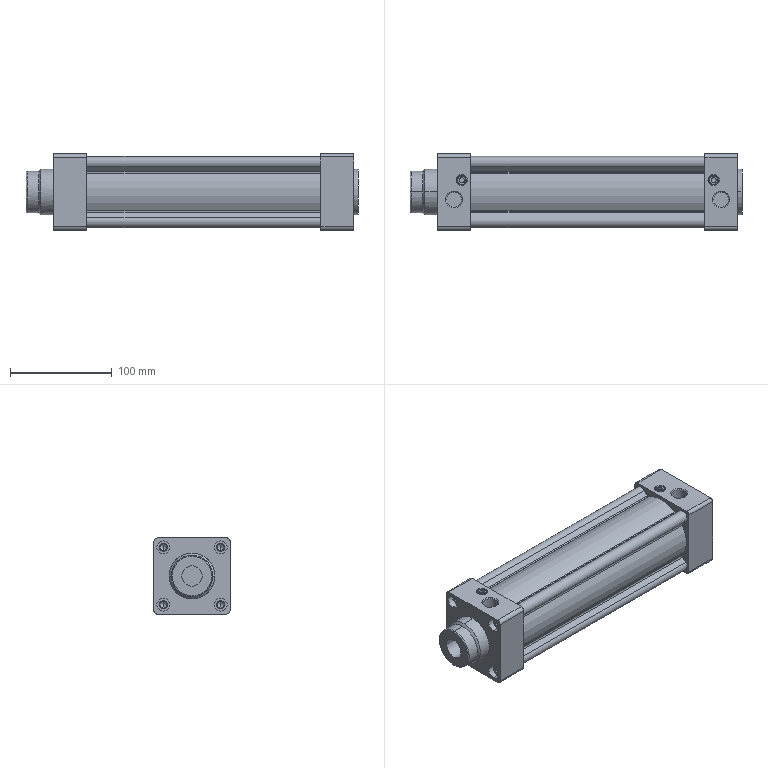Part | SolidWorks | features BaseBody 1 | 1 solid | 209 faces | box 327 x 75 x 75 mm | volume 622410 mm3 | cylinder 99 | plane 58 | cone 50 | spline 2 | commonest cylinder face diameters 6.647 x16 12.7 x16 4 x10 6.8 x8 7 x6 12 x6